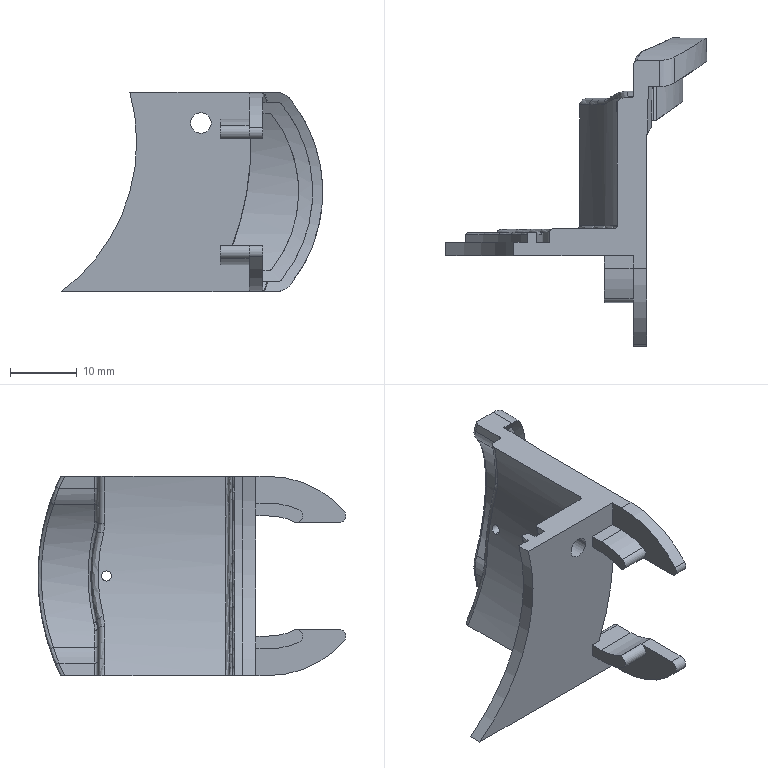Part | STEP file | ZXW722-L-13 | 1 solid | 107 faces | box 39.088 x 46.093 x 29.8 mm | volume 5108 mm3 | cylinder 51 | plane 31 | spline 11 | torus 10 | cone 4 | commonest cylinder face diameters 2 x10 1 x6 10 x4 50 x3 0.4 x2 1.5 x2